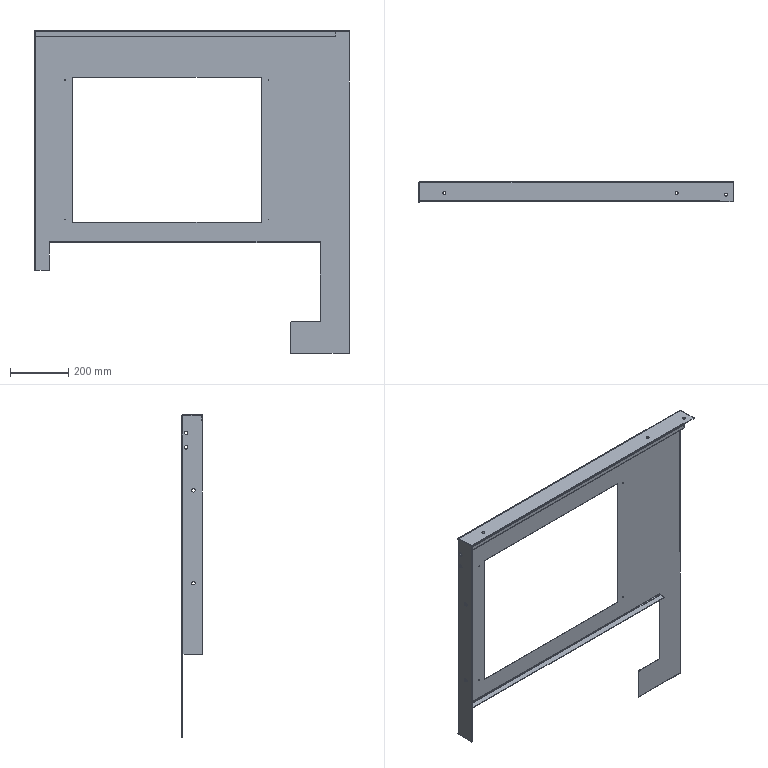Part | NX | features solid 2 | 1 solid | 71 faces | box 1083 x 70 x 1110 mm | volume 1363016 mm3 | plane 40 | cylinder 31 | commonest cylinder face diameters 2.5 x8 12 x8 4 x4 8 x4 10 x4 10.2 x2